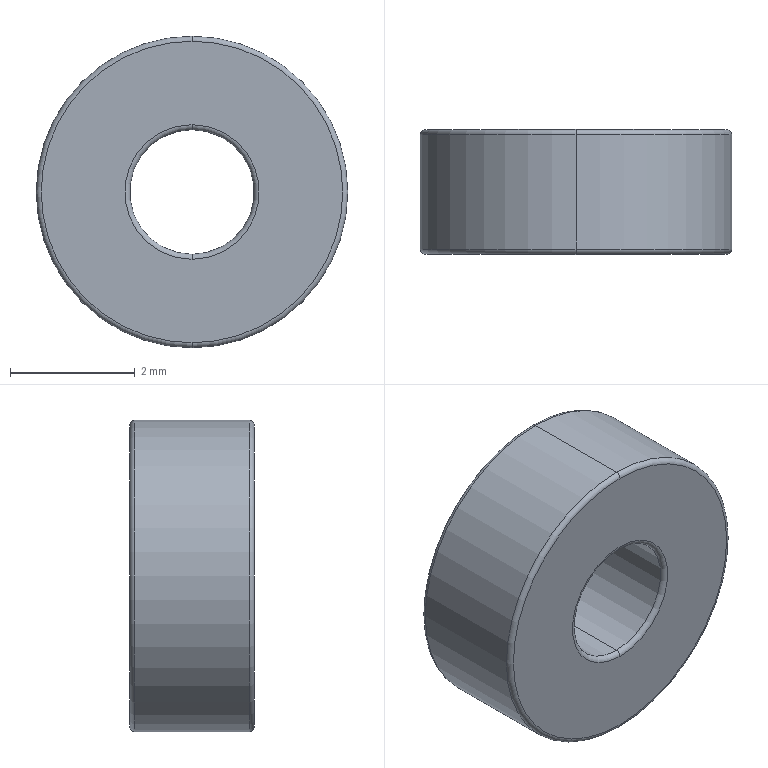Part | SolidWorks | features Extrusion 1, Fillet 1 | 1 solid | 14 faces | box 5 x 2 x 5 mm | volume 32.926 mm3 | torus 8 | cylinder 4 | plane 2 | commonest cylinder face diameters 2 x2 5 x2
STEP:
#1=CARTESIAN_POINT('',(0.,2.,-1.08));
#2=VERTEX_POINT('',#1);
#3=CARTESIAN_POINT('',(0.,2.,1.08));
#4=VERTEX_POINT('',#3);
#5=CARTESIAN_POINT('',(0.,2.,0.));
#6=DIRECTION('',(0.,-1.,0.));
#7=DIRECTION('',(0.,0.,1.));
#8=AXIS2_PLACEMENT_3D('',#5,#6,#7);
#9=CIRCLE('',#8,1.08);
#10=EDGE_CURVE('',#2,#4,#9,.T.);
#11=ORIENTED_EDGE('',*,*,#10,.F.);
#12=CARTESIAN_POINT('',(0.,1.92,-1.));
#13=VERTEX_POINT('',#12);
#14=CARTESIAN_POINT('',(0.,1.92,-1.08));
#15=DIRECTION('',(1.,0.,0.));
#16=DIRECTION('',(0.,0.,-1.));
#17=AXIS2_PLACEMENT_3D('',#14,#15,#16);
#18=CIRCLE('',#17,0.08);
#19=EDGE_CURVE('',#2,#13,#18,.T.);
#20=ORIENTED_EDGE('',*,*,#19,.T.);
#21=CARTESIAN_POINT('',(0.,1.92,1.));
#22=VERTEX_POINT('',#21);
#23=CARTESIAN_POINT('',(0.,1.92,0.));
#24=DIRECTION('',(0.,1.,0.));
#25=DIRECTION('',(0.,0.,1.));
#26=AXIS2_PLACEMENT_3D('',#23,#24,#25);
#27=CIRCLE('',#26,1.);
#28=EDGE_CURVE('',#22,#13,#27,.T.);
#29=ORIENTED_EDGE('',*,*,#28,.F.);
#30=CARTESIAN_POINT('',(0.,1.92,1.08));
#31=DIRECTION('',(-1.,0.,0.));
#32=DIRECTION('',(0.,0.,1.));
#33=AXIS2_PLACEMENT_3D('',#30,#31,#32);
#34=CIRCLE('',#33,0.08);
#35=EDGE_CURVE('',#4,#22,#34,.T.);
#36=ORIENTED_EDGE('',*,*,#35,.F.);
#37=EDGE_LOOP('',(#11,#20,#29,#36));
#38=FACE_OUTER_BOUND('',#37,.T.);
#39=CARTESIAN_POINT('',(0.,1.92,0.));
#40=DIRECTION('',(0.,1.,0.));
#41=DIRECTION('',(0.,0.,1.));
#42=AXIS2_PLACEMENT_3D('',#39,#40,#41);
#43=TOROIDAL_SURFACE('',#42,1.08,0.08);
#44=ADVANCED_FACE('',(#38),#43,.T.);
#45=CARTESIAN_POINT('',(0.,0.08,-1.));
#46=VERTEX_POINT('',#45);
#47=CARTESIAN_POINT('',(0.,0.08,1.));
#48=VERTEX_POINT('',#47);
#49=CARTESIAN_POINT('',(0.,0.08,0.));
#50=DIRECTION('',(0.,-1.,0.));
#51=DIRECTION('',(0.,0.,1.));
#52=AXIS2_PLACEMENT_3D('',#49,#50,#51);
#53=CIRCLE('',#52,1.);
#54=EDGE_CURVE('',#46,#48,#53,.T.);
#55=ORIENTED_EDGE('',*,*,#54,.F.);
#56=CARTESIAN_POINT('',(0.,0.,-1.08));
#57=VERTEX_POINT('',#56);
#58=CARTESIAN_POINT('',(0.,0.08,-1.08));
#59=DIRECTION('',(1.,0.,0.));
#60=DIRECTION('',(0.,0.,-1.));
#61=AXIS2_PLACEMENT_3D('',#58,#59,#60);
#62=CIRCLE('',#61,0.08);
#63=EDGE_CURVE('',#46,#57,#62,.T.);
#64=ORIENTED_EDGE('',*,*,#63,.T.);
#65=CARTESIAN_POINT('',(0.,0.,1.08));
#66=VERTEX_POINT('',#65);
#67=CARTESIAN_POINT('',(0.,0.,0.));
#68=DIRECTION('',(0.,1.,0.));
#69=DIRECTION('',(0.,0.,1.));
#70=AXIS2_PLACEMENT_3D('',#67,#68,#69);
#71=CIRCLE('',#70,1.08);
#72=EDGE_CURVE('',#66,#57,#71,.T.);
#73=ORIENTED_EDGE('',*,*,#72,.F.);
#74=CARTESIAN_POINT('',(0.,0.08,1.08));
#75=DIRECTION('',(-1.,0.,0.));
#76=DIRECTION('',(0.,0.,1.));
#77=AXIS2_PLACEMENT_3D('',#74,#75,#76);
#78=CIRCLE('',#77,0.08);
#79=EDGE_CURVE('',#48,#66,#78,.T.);
#80=ORIENTED_EDGE('',*,*,#79,.F.);
#81=EDGE_LOOP('',(#55,#64,#73,#80));
#82=FACE_OUTER_BOUND('',#81,.T.);
#83=CARTESIAN_POINT('',(0.,0.08,0.));
#84=DIRECTION('',(0.,1.,0.));
#85=DIRECTION('',(0.,0.,1.));
#86=AXIS2_PLACEMENT_3D('',#83,#84,#85);
#87=TOROIDAL_SURFACE('',#86,1.08,0.08);
#88=ADVANCED_FACE('',(#82),#87,.T.);
#89=CARTESIAN_POINT('',(0.,1.92,-2.5));
#90=VERTEX_POINT('',#89);
#91=CARTESIAN_POINT('',(0.,1.92,2.5));
#92=VERTEX_POINT('',#91);
#93=CARTESIAN_POINT('',(0.,1.92,0.));
#94=DIRECTION('',(0.,-1.,0.));
#95=DIRECTION('',(0.,0.,1.));
#96=AXIS2_PLACEMENT_3D('',#93,#94,#95);
#97=CIRCLE('',#96,2.5);
#98=EDGE_CURVE('',#90,#92,#97,.T.);
#99=ORIENTED_EDGE('',*,*,#98,.F.);
#100=CARTESIAN_POINT('',(0.,2.,-2.42));
#101=VERTEX_POINT('',#100);
#102=CARTESIAN_POINT('',(0.,1.92,-2.42));
#103=DIRECTION('',(1.,0.,0.));
#104=DIRECTION('',(0.,0.,-1.));
#105=AXIS2_PLACEMENT_3D('',#102,#103,#104);
#106=CIRCLE('',#105,0.08);
#107=EDGE_CURVE('',#90,#101,#106,.T.);
#108=ORIENTED_EDGE('',*,*,#107,.T.);
#109=CARTESIAN_POINT('',(0.,2.,2.42));
#110=VERTEX_POINT('',#109);
#111=CARTESIAN_POINT('',(0.,2.,0.));
#112=DIRECTION('',(0.,1.,0.));
#113=DIRECTION('',(0.,0.,1.));
#114=AXIS2_PLACEMENT_3D('',#111,#112,#113);
#115=CIRCLE('',#114,2.42);
#116=EDGE_CURVE('',#110,#101,#115,.T.);
#117=ORIENTED_EDGE('',*,*,#116,.F.);
#118=CARTESIAN_POINT('',(0.,1.92,2.42));
#119=DIRECTION('',(-1.,0.,0.));
#120=DIRECTION('',(0.,0.,1.));
#121=AXIS2_PLACEMENT_3D('',#118,#119,#120);
#122=CIRCLE('',#121,0.08);
#123=EDGE_CURVE('',#92,#110,#122,.T.);
#124=ORIENTED_EDGE('',*,*,#123,.F.);
#125=EDGE_LOOP('',(#99,#108,#117,#124));
#126=FACE_OUTER_BOUND('',#125,.T.);
#127=CARTESIAN_POINT('',(0.,1.92,0.));
#128=DIRECTION('',(0.,1.,0.));
#129=DIRECTION('',(0.,0.,1.));
#130=AXIS2_PLACEMENT_3D('',#127,#128,#129);
#131=TOROIDAL_SURFACE('',#130,2.42,0.08);
#132=ADVANCED_FACE('',(#126),#131,.T.);
#133=CARTESIAN_POINT('',(0.,0.,-2.42));
#134=VERTEX_POINT('',#133);
#135=CARTESIAN_POINT('',(0.,0.,2.42));
#136=VERTEX_POINT('',#135);
#137=CARTESIAN_POINT('',(0.,0.,0.));
#138=DIRECTION('',(0.,-1.,0.));
#139=DIRECTION('',(0.,0.,1.));
#140=AXIS2_PLACEMENT_3D('',#137,#138,#139);
#141=CIRCLE('',#140,2.42);
#142=EDGE_CURVE('',#134,#136,#141,.T.);
#143=ORIENTED_EDGE('',*,*,#142,.F.);
#144=CARTESIAN_POINT('',(0.,0.08,-2.5));
#145=VERTEX_POINT('',#144);
#146=CARTESIAN_POINT('',(0.,0.08,-2.42));
#147=DIRECTION('',(1.,0.,0.));
#148=DIRECTION('',(0.,0.,-1.));
#149=AXIS2_PLACEMENT_3D('',#146,#147,#148);
#150=CIRCLE('',#149,0.08);
#151=EDGE_CURVE('',#134,#145,#150,.T.);
#152=ORIENTED_EDGE('',*,*,#151,.T.);
#153=CARTESIAN_POINT('',(0.,0.08,2.5));
#154=VERTEX_POINT('',#153);
#155=CARTESIAN_POINT('',(0.,0.08,0.));
#156=DIRECTION('',(0.,1.,0.));
#157=DIRECTION('',(0.,0.,1.));
#158=AXIS2_PLACEMENT_3D('',#155,#156,#157);
#159=CIRCLE('',#158,2.5);
#160=EDGE_CURVE('',#154,#145,#159,.T.);
#161=ORIENTED_EDGE('',*,*,#160,.F.);
#162=CARTESIAN_POINT('',(0.,0.08,2.42));
#163=DIRECTION('',(-1.,0.,0.));
#164=DIRECTION('',(0.,0.,1.));
#165=AXIS2_PLACEMENT_3D('',#162,#163,#164);
#166=CIRCLE('',#165,0.08);
#167=EDGE_CURVE('',#136,#154,#166,.T.);
#168=ORIENTED_EDGE('',*,*,#167,.F.);
#169=EDGE_LOOP('',(#143,#152,#161,#168));
#170=FACE_OUTER_BOUND('',#169,.T.);
#171=CARTESIAN_POINT('',(0.,0.08,0.));
#172=DIRECTION('',(0.,1.,0.));
#173=DIRECTION('',(0.,0.,1.));
#174=AXIS2_PLACEMENT_3D('',#171,#172,#173);
#175=TOROIDAL_SURFACE('',#174,2.42,0.08);
#176=ADVANCED_FACE('',(#170),#175,.T.);
#177=CARTESIAN_POINT('',(0.,1.92,0.));
#178=DIRECTION('',(0.,1.,0.));
#179=DIRECTION('',(0.,0.,1.));
#180=AXIS2_PLACEMENT_3D('',#177,#178,#179);
#181=CIRCLE('',#180,1.);
#182=EDGE_CURVE('',#13,#22,#181,.T.);
#183=ORIENTED_EDGE('',*,*,#182,.T.);
#184=CARTESIAN_POINT('',(0.,2.,1.));
#185=DIRECTION('',(0.,-1.,0.));
#186=VECTOR('',#185,1000.);
#187=LINE('',#184,#186);
#188=EDGE_CURVE('',#22,#48,#187,.T.);
#189=ORIENTED_EDGE('',*,*,#188,.T.);
#190=CARTESIAN_POINT('',(0.,0.08,0.));
#191=DIRECTION('',(0.,-1.,0.));
#192=DIRECTION('',(0.,0.,1.));
#193=AXIS2_PLACEMENT_3D('',#190,#191,#192);
#194=CIRCLE('',#193,1.);
#195=EDGE_CURVE('',#48,#46,#194,.T.);
#196=ORIENTED_EDGE('',*,*,#195,.T.);
#197=CARTESIAN_POINT('',(0.,2.,-1.));
#198=DIRECTION('',(0.,-1.,0.));
#199=VECTOR('',#198,1000.);
#200=LINE('',#197,#199);
#201=EDGE_CURVE('',#13,#46,#200,.T.);
#202=ORIENTED_EDGE('',*,*,#201,.F.);
#203=EDGE_LOOP('',(#183,#189,#196,#202));
#204=FACE_OUTER_BOUND('',#203,.T.);
#205=CARTESIAN_POINT('',(0.,2.,0.));
#206=DIRECTION('',(0.,-1.,0.));
#207=DIRECTION('',(0.,0.,-1.));
#208=AXIS2_PLACEMENT_3D('',#205,#206,#207);
#209=CYLINDRICAL_SURFACE('',#208,1.);
#210=ADVANCED_FACE('',(#204),#209,.F.);
#211=ORIENTED_EDGE('',*,*,#98,.T.);
#212=CARTESIAN_POINT('',(0.,2.,2.5));
#213=DIRECTION('',(0.,-1.,0.));
#214=VECTOR('',#213,1000.);
#215=LINE('',#212,#214);
#216=EDGE_CURVE('',#92,#154,#215,.T.);
#217=ORIENTED_EDGE('',*,*,#216,.T.);
#218=ORIENTED_EDGE('',*,*,#160,.T.);
#219=CARTESIAN_POINT('',(0.,2.,-2.5));
#220=DIRECTION('',(0.,-1.,0.));
#221=VECTOR('',#220,1000.);
#222=LINE('',#219,#221);
#223=EDGE_CURVE('',#90,#145,#222,.T.);
#224=ORIENTED_EDGE('',*,*,#223,.F.);
#225=EDGE_LOOP('',(#211,#217,#218,#224));
#226=FACE_OUTER_BOUND('',#225,.T.);
#227=CARTESIAN_POINT('',(0.,2.,0.));
#228=DIRECTION('',(0.,-1.,0.));
#229=DIRECTION('',(0.,0.,-1.));
#230=AXIS2_PLACEMENT_3D('',#227,#228,#229);
#231=CYLINDRICAL_SURFACE('',#230,2.5);
#232=ADVANCED_FACE('',(#226),#231,.T.);
#233=ORIENTED_EDGE('',*,*,#116,.T.);
#234=CARTESIAN_POINT('',(0.,2.,0.));
#235=DIRECTION('',(0.,1.,0.));
#236=DIRECTION('',(0.,0.,1.));
#237=AXIS2_PLACEMENT_3D('',#234,#235,#236);
#238=CIRCLE('',#237,2.42);
#239=EDGE_CURVE('',#101,#110,#238,.T.);
#240=ORIENTED_EDGE('',*,*,#239,.T.);
#241=EDGE_LOOP('',(#233,#240));
#242=FACE_OUTER_BOUND('',#241,.T.);
#243=CARTESIAN_POINT('',(0.,2.,0.));
#244=DIRECTION('',(0.,-1.,0.));
#245=DIRECTION('',(0.,0.,1.));
#246=AXIS2_PLACEMENT_3D('',#243,#244,#245);
#247=CIRCLE('',#246,1.08);
#248=EDGE_CURVE('',#4,#2,#247,.T.);
#249=ORIENTED_EDGE('',*,*,#248,.T.);
#250=ORIENTED_EDGE('',*,*,#10,.T.);
#251=EDGE_LOOP('',(#249,#250));
#252=FACE_BOUND('',#251,.T.);
#253=CARTESIAN_POINT('',(0.,2.,0.));
#254=DIRECTION('',(0.,1.,0.));
#255=DIRECTION('',(0.,0.,1.));
#256=AXIS2_PLACEMENT_3D('',#253,#254,#255);
#257=PLANE('',#256);
#258=ADVANCED_FACE('',(#242,#252),#257,.T.);
#259=CARTESIAN_POINT('',(0.,0.,0.));
#260=DIRECTION('',(0.,-1.,0.));
#261=DIRECTION('',(0.,0.,1.));
#262=AXIS2_PLACEMENT_3D('',#259,#260,#261);
#263=CIRCLE('',#262,2.42);
#264=EDGE_CURVE('',#136,#134,#263,.T.);
#265=ORIENTED_EDGE('',*,*,#264,.T.);
#266=ORIENTED_EDGE('',*,*,#142,.T.);
#267=EDGE_LOOP('',(#265,#266));
#268=FACE_OUTER_BOUND('',#267,.T.);
#269=ORIENTED_EDGE('',*,*,#72,.T.);
#270=CARTESIAN_POINT('',(0.,0.,0.));
#271=DIRECTION('',(0.,1.,0.));
#272=DIRECTION('',(0.,0.,1.));
#273=AXIS2_PLACEMENT_3D('',#270,#271,#272);
#274=CIRCLE('',#273,1.08);
#275=EDGE_CURVE('',#57,#66,#274,.T.);
#276=ORIENTED_EDGE('',*,*,#275,.T.);
#277=EDGE_LOOP('',(#269,#276));
#278=FACE_BOUND('',#277,.T.);
#279=CARTESIAN_POINT('',(0.,0.,0.));
#280=DIRECTION('',(0.,1.,0.));
#281=DIRECTION('',(0.,0.,1.));
#282=AXIS2_PLACEMENT_3D('',#279,#280,#281);
#283=PLANE('',#282);
#284=ADVANCED_FACE('',(#268,#278),#283,.F.);
#285=ORIENTED_EDGE('',*,*,#216,.F.);
#286=CARTESIAN_POINT('',(0.,1.92,0.));
#287=DIRECTION('',(0.,-1.,0.));
#288=DIRECTION('',(0.,0.,1.));
#289=AXIS2_PLACEMENT_3D('',#286,#287,#288);
#290=CIRCLE('',#289,2.5);
#291=EDGE_CURVE('',#92,#90,#290,.T.);
#292=ORIENTED_EDGE('',*,*,#291,.T.);
#293=ORIENTED_EDGE('',*,*,#223,.T.);
#294=CARTESIAN_POINT('',(0.,0.08,0.));
#295=DIRECTION('',(0.,1.,0.));
#296=DIRECTION('',(0.,0.,1.));
#297=AXIS2_PLACEMENT_3D('',#294,#295,#296);
#298=CIRCLE('',#297,2.5);
#299=EDGE_CURVE('',#145,#154,#298,.T.);
#300=ORIENTED_EDGE('',*,*,#299,.T.);
#301=EDGE_LOOP('',(#285,#292,#293,#300));
#302=FACE_OUTER_BOUND('',#301,.T.);
#303=CARTESIAN_POINT('',(0.,2.,0.));
#304=DIRECTION('',(0.,-1.,0.));
#305=DIRECTION('',(0.,0.,-1.));
#306=AXIS2_PLACEMENT_3D('',#303,#304,#305);
#307=CYLINDRICAL_SURFACE('',#306,2.5);
#308=ADVANCED_FACE('',(#302),#307,.T.);
#309=ORIENTED_EDGE('',*,*,#188,.F.);
#310=ORIENTED_EDGE('',*,*,#28,.T.);
#311=ORIENTED_EDGE('',*,*,#201,.T.);
#312=ORIENTED_EDGE('',*,*,#54,.T.);
#313=EDGE_LOOP('',(#309,#310,#311,#312));
#314=FACE_OUTER_BOUND('',#313,.T.);
#315=CARTESIAN_POINT('',(0.,2.,0.));
#316=DIRECTION('',(0.,-1.,0.));
#317=DIRECTION('',(0.,0.,-1.));
#318=AXIS2_PLACEMENT_3D('',#315,#316,#317);
#319=CYLINDRICAL_SURFACE('',#318,1.);
#320=ADVANCED_FACE('',(#314),#319,.F.);
#321=ORIENTED_EDGE('',*,*,#151,.F.);
#322=ORIENTED_EDGE('',*,*,#264,.F.);
#323=ORIENTED_EDGE('',*,*,#167,.T.);
#324=ORIENTED_EDGE('',*,*,#299,.F.);
#325=EDGE_LOOP('',(#321,#322,#323,#324));
#326=FACE_OUTER_BOUND('',#325,.T.);
#327=CARTESIAN_POINT('',(0.,0.08,0.));
#328=DIRECTION('',(0.,1.,0.));
#329=DIRECTION('',(0.,0.,1.));
#330=AXIS2_PLACEMENT_3D('',#327,#328,#329);
#331=TOROIDAL_SURFACE('',#330,2.42,0.08);
#332=ADVANCED_FACE('',(#326),#331,.T.);
#333=ORIENTED_EDGE('',*,*,#107,.F.);
#334=ORIENTED_EDGE('',*,*,#291,.F.);
#335=ORIENTED_EDGE('',*,*,#123,.T.);
#336=ORIENTED_EDGE('',*,*,#239,.F.);
#337=EDGE_LOOP('',(#333,#334,#335,#336));
#338=FACE_OUTER_BOUND('',#337,.T.);
#339=CARTESIAN_POINT('',(0.,1.92,0.));
#340=DIRECTION('',(0.,1.,0.));
#341=DIRECTION('',(0.,0.,1.));
#342=AXIS2_PLACEMENT_3D('',#339,#340,#341);
#343=TOROIDAL_SURFACE('',#342,2.42,0.08);
#344=ADVANCED_FACE('',(#338),#343,.T.);
#345=ORIENTED_EDGE('',*,*,#63,.F.);
#346=ORIENTED_EDGE('',*,*,#195,.F.);
#347=ORIENTED_EDGE('',*,*,#79,.T.);
#348=ORIENTED_EDGE('',*,*,#275,.F.);
#349=EDGE_LOOP('',(#345,#346,#347,#348));
#350=FACE_OUTER_BOUND('',#349,.T.);
#351=CARTESIAN_POINT('',(0.,0.08,0.));
#352=DIRECTION('',(0.,1.,0.));
#353=DIRECTION('',(0.,0.,1.));
#354=AXIS2_PLACEMENT_3D('',#351,#352,#353);
#355=TOROIDAL_SURFACE('',#354,1.08,0.08);
#356=ADVANCED_FACE('',(#350),#355,.T.);
#357=ORIENTED_EDGE('',*,*,#19,.F.);
#358=ORIENTED_EDGE('',*,*,#248,.F.);
#359=ORIENTED_EDGE('',*,*,#35,.T.);
#360=ORIENTED_EDGE('',*,*,#182,.F.);
#361=EDGE_LOOP('',(#357,#358,#359,#360));
#362=FACE_OUTER_BOUND('',#361,.T.);
#363=CARTESIAN_POINT('',(0.,1.92,0.));
#364=DIRECTION('',(0.,1.,0.));
#365=DIRECTION('',(0.,0.,1.));
#366=AXIS2_PLACEMENT_3D('',#363,#364,#365);
#367=TOROIDAL_SURFACE('',#366,1.08,0.08);
#368=ADVANCED_FACE('',(#362),#367,.T.);
#369=CLOSED_SHELL('',(#44,#88,#132,#176,#210,#232,#258,#284,#308,#320,#332,#344,#356,#368));
#370=MANIFOLD_SOLID_BREP('',#369);
#371=CARTESIAN_POINT('',(0.,0.,0.));
#372=DIRECTION('',(0.,0.,1.));
#373=DIRECTION('',(1.,0.,0.));
#374=AXIS2_PLACEMENT_3D('',#371,#372,#373);
#375=(LENGTH_UNIT()NAMED_UNIT(*)SI_UNIT(.MILLI.,.METRE.));
#376=UNCERTAINTY_MEASURE_WITH_UNIT(LENGTH_MEASURE(0.00001),#375,'','');
#377=(NAMED_UNIT(*)PLANE_ANGLE_UNIT()SI_UNIT($,.RADIAN.));
#378=(NAMED_UNIT(*)SI_UNIT($,.STERADIAN.)SOLID_ANGLE_UNIT());
#379=(GEOMETRIC_REPRESENTATION_CONTEXT(3)GLOBAL_UNCERTAINTY_ASSIGNED_CONTEXT((#376))GLOBAL_UNIT_ASSIGNED_CONTEXT((#375,#377,#378))REPRESENTATION_CONTEXT('',''));
#380=ADVANCED_BREP_SHAPE_REPRESENTATION('',(#370,#374),#379);